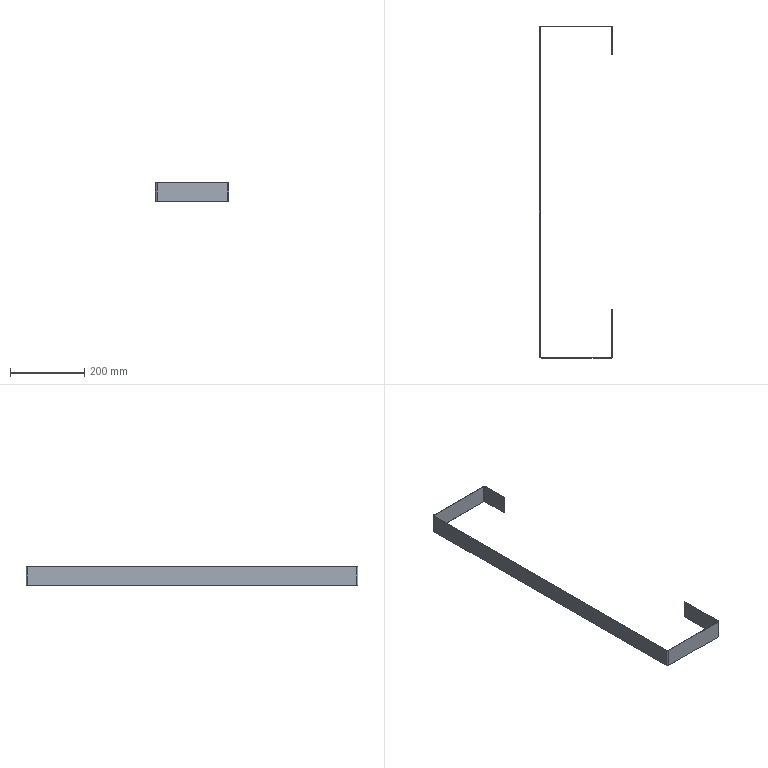Part | STEP file | Connector | 1 solid | 22 faces | box 197.5 x 897 x 50 mm | volume 111605 mm3 | plane 14 | cylinder 8 | commonest cylinder face diameters 4 x2 6 x2 7 x2 10 x2